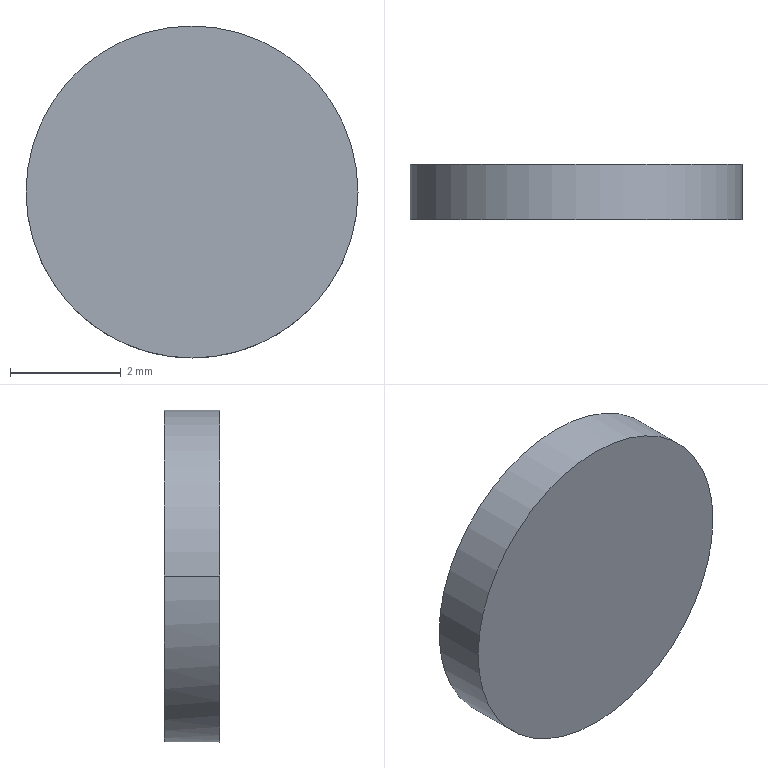Part | Creo | 1 solid | 17 faces | box 6 x 1 x 6 mm | volume 26.294 mm3 | plane 15 | cylinder 2 | commonest cylinder face diameters 6 x2
STEP:
#1=CARTESIAN_POINT('',(0.,0.,0.));
#2=DIRECTION('',(0.,0.,1.));
#3=DIRECTION('',(1.,0.,0.));
#4=AXIS2_PLACEMENT_3D('',#1,#2,#3);
#5=CARTESIAN_POINT('',(58.,52.,60.91));
#6=VERTEX_POINT('',#5);
#7=CARTESIAN_POINT('',(55.,52.,63.91));
#8=VERTEX_POINT('',#7);
#9=CARTESIAN_POINT('',(55.,52.,60.91));
#10=DIRECTION('',(0.,-1.,0.));
#11=DIRECTION('',(1.,0.,0.));
#12=AXIS2_PLACEMENT_3D('',#9,#10,#11);
#13=CIRCLE('',#12,3.);
#14=EDGE_CURVE('',#6,#8,#13,.T.);
#15=ORIENTED_EDGE('',*,*,#14,.T.);
#16=CARTESIAN_POINT('',(52.,52.,60.91));
#17=VERTEX_POINT('',#16);
#18=CARTESIAN_POINT('',(55.,52.,60.91));
#19=DIRECTION('',(0.,-1.,0.));
#20=DIRECTION('',(0.,0.,1.));
#21=AXIS2_PLACEMENT_3D('',#18,#19,#20);
#22=CIRCLE('',#21,3.);
#23=EDGE_CURVE('',#8,#17,#22,.T.);
#24=ORIENTED_EDGE('',*,*,#23,.T.);
#25=CARTESIAN_POINT('',(52.,53.,60.91));
#26=VERTEX_POINT('',#25);
#27=CARTESIAN_POINT('',(52.,52.,60.91));
#28=DIRECTION('',(0.,1.,0.));
#29=VECTOR('',#28,1.);
#30=LINE('',#27,#29);
#31=EDGE_CURVE('',#17,#26,#30,.T.);
#32=ORIENTED_EDGE('',*,*,#31,.T.);
#33=CARTESIAN_POINT('',(55.,53.,63.91));
#34=VERTEX_POINT('',#33);
#35=CARTESIAN_POINT('',(55.,53.,60.91));
#36=DIRECTION('',(0.,1.,0.));
#37=DIRECTION('',(-1.,0.,0.));
#38=AXIS2_PLACEMENT_3D('',#35,#36,#37);
#39=CIRCLE('',#38,3.);
#40=EDGE_CURVE('',#26,#34,#39,.T.);
#41=ORIENTED_EDGE('',*,*,#40,.T.);
#42=CARTESIAN_POINT('',(58.,53.,60.91));
#43=VERTEX_POINT('',#42);
#44=CARTESIAN_POINT('',(55.,53.,60.91));
#45=DIRECTION('',(0.,1.,0.));
#46=DIRECTION('',(0.,0.,1.));
#47=AXIS2_PLACEMENT_3D('',#44,#45,#46);
#48=CIRCLE('',#47,3.);
#49=EDGE_CURVE('',#34,#43,#48,.T.);
#50=ORIENTED_EDGE('',*,*,#49,.T.);
#51=CARTESIAN_POINT('',(58.,52.,60.91));
#52=DIRECTION('',(0.,1.,0.));
#53=VECTOR('',#52,1.);
#54=LINE('',#51,#53);
#55=EDGE_CURVE('',#6,#43,#54,.T.);
#56=ORIENTED_EDGE('',*,*,#55,.F.);
#57=EDGE_LOOP('',(#15,#24,#32,#41,#50,#56));
#58=FACE_OUTER_BOUND('',#57,.F.);
#59=CARTESIAN_POINT('',(55.,52.,60.91));
#60=DIRECTION('',(0.,1.,0.));
#61=DIRECTION('',(-1.,0.,0.));
#62=AXIS2_PLACEMENT_3D('',#59,#60,#61);
#63=CYLINDRICAL_SURFACE('',#62,3.);
#64=ADVANCED_FACE('',(#58),#63,.T.);
#65=ORIENTED_EDGE('',*,*,#23,.F.);
#66=ORIENTED_EDGE('',*,*,#14,.F.);
#67=CARTESIAN_POINT('',(55.,52.,57.91));
#68=VERTEX_POINT('',#67);
#69=CARTESIAN_POINT('',(55.,52.,60.91));
#70=DIRECTION('',(0.,-1.,0.));
#71=DIRECTION('',(0.,0.,-1.));
#72=AXIS2_PLACEMENT_3D('',#69,#70,#71);
#73=CIRCLE('',#72,3.);
#74=EDGE_CURVE('',#68,#6,#73,.T.);
#75=ORIENTED_EDGE('',*,*,#74,.F.);
#76=CARTESIAN_POINT('',(55.,52.,60.91));
#77=DIRECTION('',(0.,-1.,0.));
#78=DIRECTION('',(-1.,0.,0.));
#79=AXIS2_PLACEMENT_3D('',#76,#77,#78);
#80=CIRCLE('',#79,3.);
#81=EDGE_CURVE('',#17,#68,#80,.T.);
#82=ORIENTED_EDGE('',*,*,#81,.F.);
#83=EDGE_LOOP('',(#65,#66,#75,#82));
#84=FACE_OUTER_BOUND('',#83,.F.);
#85=CARTESIAN_POINT('',(55.,52.,60.91));
#86=DIRECTION('',(0.,-1.,0.));
#87=DIRECTION('',(1.,0.,0.));
#88=AXIS2_PLACEMENT_3D('',#85,#86,#87);
#89=PLANE('',#88);
#90=ADVANCED_FACE('',(#84),#89,.T.);
#91=ORIENTED_EDGE('',*,*,#74,.T.);
#92=ORIENTED_EDGE('',*,*,#55,.T.);
#93=CARTESIAN_POINT('',(55.,53.,60.91));
#94=DIRECTION('',(0.,1.,0.));
#95=DIRECTION('',(1.,0.,0.));
#96=AXIS2_PLACEMENT_3D('',#93,#94,#95);
#97=CIRCLE('',#96,3.);
#98=EDGE_CURVE('',#43,#26,#97,.T.);
#99=ORIENTED_EDGE('',*,*,#98,.T.);
#100=ORIENTED_EDGE('',*,*,#31,.F.);
#101=ORIENTED_EDGE('',*,*,#81,.T.);
#102=EDGE_LOOP('',(#91,#92,#99,#100,#101));
#103=FACE_OUTER_BOUND('',#102,.F.);
#104=CARTESIAN_POINT('',(55.,52.,60.91));
#105=DIRECTION('',(0.,1.,0.));
#106=DIRECTION('',(-1.,0.,0.));
#107=AXIS2_PLACEMENT_3D('',#104,#105,#106);
#108=CYLINDRICAL_SURFACE('',#107,3.);
#109=ADVANCED_FACE('',(#103),#108,.T.);
#110=ORIENTED_EDGE('',*,*,#49,.F.);
#111=ORIENTED_EDGE('',*,*,#40,.F.);
#112=ORIENTED_EDGE('',*,*,#98,.F.);
#113=EDGE_LOOP('',(#110,#111,#112));
#114=FACE_OUTER_BOUND('',#113,.F.);
#115=CARTESIAN_POINT('',(53.2,53.,61.21));
#116=VERTEX_POINT('',#115);
#117=CARTESIAN_POINT('',(54.7,53.,61.21));
#118=VERTEX_POINT('',#117);
#119=CARTESIAN_POINT('',(53.2,53.,61.21));
#120=DIRECTION('',(1.,0.,0.));
#121=VECTOR('',#120,1.5);
#122=LINE('',#119,#121);
#123=EDGE_CURVE('',#116,#118,#122,.T.);
#124=ORIENTED_EDGE('',*,*,#123,.T.);
#125=CARTESIAN_POINT('',(54.7,53.,62.71));
#126=VERTEX_POINT('',#125);
#127=CARTESIAN_POINT('',(54.7,53.,61.21));
#128=DIRECTION('',(0.,0.,1.));
#129=VECTOR('',#128,1.5);
#130=LINE('',#127,#129);
#131=EDGE_CURVE('',#118,#126,#130,.T.);
#132=ORIENTED_EDGE('',*,*,#131,.T.);
#133=CARTESIAN_POINT('',(55.3,53.,62.71));
#134=VERTEX_POINT('',#133);
#135=CARTESIAN_POINT('',(54.7,53.,62.71));
#136=DIRECTION('',(1.,0.,0.));
#137=VECTOR('',#136,0.6);
#138=LINE('',#135,#137);
#139=EDGE_CURVE('',#126,#134,#138,.T.);
#140=ORIENTED_EDGE('',*,*,#139,.T.);
#141=CARTESIAN_POINT('',(55.3,53.,61.21));
#142=VERTEX_POINT('',#141);
#143=CARTESIAN_POINT('',(55.3,53.,62.71));
#144=DIRECTION('',(0.,0.,-1.));
#145=VECTOR('',#144,1.5);
#146=LINE('',#143,#145);
#147=EDGE_CURVE('',#134,#142,#146,.T.);
#148=ORIENTED_EDGE('',*,*,#147,.T.);
#149=CARTESIAN_POINT('',(56.8,53.,61.21));
#150=VERTEX_POINT('',#149);
#151=CARTESIAN_POINT('',(55.3,53.,61.21));
#152=DIRECTION('',(1.,0.,0.));
#153=VECTOR('',#152,1.5);
#154=LINE('',#151,#153);
#155=EDGE_CURVE('',#142,#150,#154,.T.);
#156=ORIENTED_EDGE('',*,*,#155,.T.);
#157=CARTESIAN_POINT('',(56.8,53.,60.61));
#158=VERTEX_POINT('',#157);
#159=CARTESIAN_POINT('',(56.8,53.,61.21));
#160=DIRECTION('',(0.,0.,-1.));
#161=VECTOR('',#160,0.6);
#162=LINE('',#159,#161);
#163=EDGE_CURVE('',#150,#158,#162,.T.);
#164=ORIENTED_EDGE('',*,*,#163,.T.);
#165=CARTESIAN_POINT('',(55.3,53.,60.61));
#166=VERTEX_POINT('',#165);
#167=CARTESIAN_POINT('',(56.8,53.,60.61));
#168=DIRECTION('',(-1.,0.,0.));
#169=VECTOR('',#168,1.5);
#170=LINE('',#167,#169);
#171=EDGE_CURVE('',#158,#166,#170,.T.);
#172=ORIENTED_EDGE('',*,*,#171,.T.);
#173=CARTESIAN_POINT('',(55.3,53.,59.11));
#174=VERTEX_POINT('',#173);
#175=CARTESIAN_POINT('',(55.3,53.,60.61));
#176=DIRECTION('',(0.,0.,-1.));
#177=VECTOR('',#176,1.5);
#178=LINE('',#175,#177);
#179=EDGE_CURVE('',#166,#174,#178,.T.);
#180=ORIENTED_EDGE('',*,*,#179,.T.);
#181=CARTESIAN_POINT('',(54.7,53.,59.11));
#182=VERTEX_POINT('',#181);
#183=CARTESIAN_POINT('',(55.3,53.,59.11));
#184=DIRECTION('',(-1.,0.,0.));
#185=VECTOR('',#184,0.6);
#186=LINE('',#183,#185);
#187=EDGE_CURVE('',#174,#182,#186,.T.);
#188=ORIENTED_EDGE('',*,*,#187,.T.);
#189=CARTESIAN_POINT('',(54.7,53.,60.61));
#190=VERTEX_POINT('',#189);
#191=CARTESIAN_POINT('',(54.7,53.,59.11));
#192=DIRECTION('',(0.,0.,1.));
#193=VECTOR('',#192,1.5);
#194=LINE('',#191,#193);
#195=EDGE_CURVE('',#182,#190,#194,.T.);
#196=ORIENTED_EDGE('',*,*,#195,.T.);
#197=CARTESIAN_POINT('',(53.2,53.,60.61));
#198=VERTEX_POINT('',#197);
#199=CARTESIAN_POINT('',(54.7,53.,60.61));
#200=DIRECTION('',(-1.,0.,0.));
#201=VECTOR('',#200,1.5);
#202=LINE('',#199,#201);
#203=EDGE_CURVE('',#190,#198,#202,.T.);
#204=ORIENTED_EDGE('',*,*,#203,.T.);
#205=CARTESIAN_POINT('',(53.2,53.,60.61));
#206=DIRECTION('',(0.,0.,1.));
#207=VECTOR('',#206,0.6);
#208=LINE('',#205,#207);
#209=EDGE_CURVE('',#198,#116,#208,.T.);
#210=ORIENTED_EDGE('',*,*,#209,.T.);
#211=EDGE_LOOP('',(#124,#132,#140,#148,#156,#164,#172,#180,#188,#196,#204,#210));
#212=FACE_BOUND('',#211,.F.);
#213=CARTESIAN_POINT('',(55.,53.,60.91));
#214=DIRECTION('',(0.,-1.,0.));
#215=DIRECTION('',(1.,0.,0.));
#216=AXIS2_PLACEMENT_3D('',#213,#214,#215);
#217=PLANE('',#216);
#218=ADVANCED_FACE('',(#114,#212),#217,.F.);
#219=ORIENTED_EDGE('',*,*,#123,.F.);
#220=CARTESIAN_POINT('',(53.2,52.5,61.21));
#221=VERTEX_POINT('',#220);
#222=CARTESIAN_POINT('',(53.2,52.5,61.21));
#223=DIRECTION('',(0.,1.,0.));
#224=VECTOR('',#223,0.5);
#225=LINE('',#222,#224);
#226=EDGE_CURVE('',#221,#116,#225,.T.);
#227=ORIENTED_EDGE('',*,*,#226,.F.);
#228=CARTESIAN_POINT('',(54.7,52.5,61.21));
#229=VERTEX_POINT('',#228);
#230=CARTESIAN_POINT('',(54.7,52.5,61.21));
#231=DIRECTION('',(-1.,0.,0.));
#232=VECTOR('',#231,1.5);
#233=LINE('',#230,#232);
#234=EDGE_CURVE('',#229,#221,#233,.T.);
#235=ORIENTED_EDGE('',*,*,#234,.F.);
#236=CARTESIAN_POINT('',(54.7,52.5,61.21));
#237=DIRECTION('',(0.,1.,0.));
#238=VECTOR('',#237,0.5);
#239=LINE('',#236,#238);
#240=EDGE_CURVE('',#229,#118,#239,.T.);
#241=ORIENTED_EDGE('',*,*,#240,.T.);
#242=EDGE_LOOP('',(#219,#227,#235,#241));
#243=FACE_OUTER_BOUND('',#242,.F.);
#244=CARTESIAN_POINT('',(54.7,52.5,61.21));
#245=DIRECTION('',(0.,0.,-1.));
#246=DIRECTION('',(-1.,0.,0.));
#247=AXIS2_PLACEMENT_3D('',#244,#245,#246);
#248=PLANE('',#247);
#249=ADVANCED_FACE('',(#243),#248,.T.);
#250=ORIENTED_EDGE('',*,*,#209,.F.);
#251=CARTESIAN_POINT('',(53.2,52.5,60.61));
#252=VERTEX_POINT('',#251);
#253=CARTESIAN_POINT('',(53.2,52.5,60.61));
#254=DIRECTION('',(0.,1.,0.));
#255=VECTOR('',#254,0.5);
#256=LINE('',#253,#255);
#257=EDGE_CURVE('',#252,#198,#256,.T.);
#258=ORIENTED_EDGE('',*,*,#257,.F.);
#259=CARTESIAN_POINT('',(53.2,52.5,61.21));
#260=DIRECTION('',(0.,0.,-1.));
#261=VECTOR('',#260,0.6);
#262=LINE('',#259,#261);
#263=EDGE_CURVE('',#221,#252,#262,.T.);
#264=ORIENTED_EDGE('',*,*,#263,.F.);
#265=ORIENTED_EDGE('',*,*,#226,.T.);
#266=EDGE_LOOP('',(#250,#258,#264,#265));
#267=FACE_OUTER_BOUND('',#266,.F.);
#268=CARTESIAN_POINT('',(53.2,52.5,61.21));
#269=DIRECTION('',(1.,0.,0.));
#270=DIRECTION('',(0.,1.,0.));
#271=AXIS2_PLACEMENT_3D('',#268,#269,#270);
#272=PLANE('',#271);
#273=ADVANCED_FACE('',(#267),#272,.T.);
#274=ORIENTED_EDGE('',*,*,#203,.F.);
#275=CARTESIAN_POINT('',(54.7,52.5,60.61));
#276=VERTEX_POINT('',#275);
#277=CARTESIAN_POINT('',(54.7,52.5,60.61));
#278=DIRECTION('',(0.,1.,0.));
#279=VECTOR('',#278,0.5);
#280=LINE('',#277,#279);
#281=EDGE_CURVE('',#276,#190,#280,.T.);
#282=ORIENTED_EDGE('',*,*,#281,.F.);
#283=CARTESIAN_POINT('',(53.2,52.5,60.61));
#284=DIRECTION('',(1.,0.,0.));
#285=VECTOR('',#284,1.5);
#286=LINE('',#283,#285);
#287=EDGE_CURVE('',#252,#276,#286,.T.);
#288=ORIENTED_EDGE('',*,*,#287,.F.);
#289=ORIENTED_EDGE('',*,*,#257,.T.);
#290=EDGE_LOOP('',(#274,#282,#288,#289));
#291=FACE_OUTER_BOUND('',#290,.F.);
#292=CARTESIAN_POINT('',(53.2,52.5,60.61));
#293=DIRECTION('',(0.,0.,1.));
#294=DIRECTION('',(1.,0.,0.));
#295=AXIS2_PLACEMENT_3D('',#292,#293,#294);
#296=PLANE('',#295);
#297=ADVANCED_FACE('',(#291),#296,.T.);
#298=ORIENTED_EDGE('',*,*,#195,.F.);
#299=CARTESIAN_POINT('',(54.7,52.5,59.11));
#300=VERTEX_POINT('',#299);
#301=CARTESIAN_POINT('',(54.7,52.5,59.11));
#302=DIRECTION('',(0.,1.,0.));
#303=VECTOR('',#302,0.5);
#304=LINE('',#301,#303);
#305=EDGE_CURVE('',#300,#182,#304,.T.);
#306=ORIENTED_EDGE('',*,*,#305,.F.);
#307=CARTESIAN_POINT('',(54.7,52.5,60.61));
#308=DIRECTION('',(0.,0.,-1.));
#309=VECTOR('',#308,1.5);
#310=LINE('',#307,#309);
#311=EDGE_CURVE('',#276,#300,#310,.T.);
#312=ORIENTED_EDGE('',*,*,#311,.F.);
#313=ORIENTED_EDGE('',*,*,#281,.T.);
#314=EDGE_LOOP('',(#298,#306,#312,#313));
#315=FACE_OUTER_BOUND('',#314,.F.);
#316=CARTESIAN_POINT('',(54.7,52.5,60.61));
#317=DIRECTION('',(1.,0.,0.));
#318=DIRECTION('',(0.,0.,-1.));
#319=AXIS2_PLACEMENT_3D('',#316,#317,#318);
#320=PLANE('',#319);
#321=ADVANCED_FACE('',(#315),#320,.T.);
#322=ORIENTED_EDGE('',*,*,#187,.F.);
#323=CARTESIAN_POINT('',(55.3,52.5,59.11));
#324=VERTEX_POINT('',#323);
#325=CARTESIAN_POINT('',(55.3,52.5,59.11));
#326=DIRECTION('',(0.,1.,0.));
#327=VECTOR('',#326,0.5);
#328=LINE('',#325,#327);
#329=EDGE_CURVE('',#324,#174,#328,.T.);
#330=ORIENTED_EDGE('',*,*,#329,.F.);
#331=CARTESIAN_POINT('',(54.7,52.5,59.11));
#332=DIRECTION('',(1.,0.,0.));
#333=VECTOR('',#332,0.6);
#334=LINE('',#331,#333);
#335=EDGE_CURVE('',#300,#324,#334,.T.);
#336=ORIENTED_EDGE('',*,*,#335,.F.);
#337=ORIENTED_EDGE('',*,*,#305,.T.);
#338=EDGE_LOOP('',(#322,#330,#336,#337));
#339=FACE_OUTER_BOUND('',#338,.F.);
#340=CARTESIAN_POINT('',(54.7,52.5,59.11));
#341=DIRECTION('',(0.,0.,1.));
#342=DIRECTION('',(0.,1.,0.));
#343=AXIS2_PLACEMENT_3D('',#340,#341,#342);
#344=PLANE('',#343);
#345=ADVANCED_FACE('',(#339),#344,.T.);
#346=ORIENTED_EDGE('',*,*,#179,.F.);
#347=CARTESIAN_POINT('',(55.3,52.5,60.61));
#348=VERTEX_POINT('',#347);
#349=CARTESIAN_POINT('',(55.3,52.5,60.61));
#350=DIRECTION('',(0.,1.,0.));
#351=VECTOR('',#350,0.5);
#352=LINE('',#349,#351);
#353=EDGE_CURVE('',#348,#166,#352,.T.);
#354=ORIENTED_EDGE('',*,*,#353,.F.);
#355=CARTESIAN_POINT('',(55.3,52.5,59.11));
#356=DIRECTION('',(0.,0.,1.));
#357=VECTOR('',#356,1.5);
#358=LINE('',#355,#357);
#359=EDGE_CURVE('',#324,#348,#358,.T.);
#360=ORIENTED_EDGE('',*,*,#359,.F.);
#361=ORIENTED_EDGE('',*,*,#329,.T.);
#362=EDGE_LOOP('',(#346,#354,#360,#361));
#363=FACE_OUTER_BOUND('',#362,.F.);
#364=CARTESIAN_POINT('',(55.3,52.5,59.11));
#365=DIRECTION('',(-1.,0.,0.));
#366=DIRECTION('',(0.,0.,1.));
#367=AXIS2_PLACEMENT_3D('',#364,#365,#366);
#368=PLANE('',#367);
#369=ADVANCED_FACE('',(#363),#368,.T.);
#370=ORIENTED_EDGE('',*,*,#171,.F.);
#371=CARTESIAN_POINT('',(56.8,52.5,60.61));
#372=VERTEX_POINT('',#371);
#373=CARTESIAN_POINT('',(56.8,52.5,60.61));
#374=DIRECTION('',(0.,1.,0.));
#375=VECTOR('',#374,0.5);
#376=LINE('',#373,#375);
#377=EDGE_CURVE('',#372,#158,#376,.T.);
#378=ORIENTED_EDGE('',*,*,#377,.F.);
#379=CARTESIAN_POINT('',(55.3,52.5,60.61));
#380=DIRECTION('',(1.,0.,0.));
#381=VECTOR('',#380,1.5);
#382=LINE('',#379,#381);
#383=EDGE_CURVE('',#348,#372,#382,.T.);
#384=ORIENTED_EDGE('',*,*,#383,.F.);
#385=ORIENTED_EDGE('',*,*,#353,.T.);
#386=EDGE_LOOP('',(#370,#378,#384,#385));
#387=FACE_OUTER_BOUND('',#386,.F.);
#388=CARTESIAN_POINT('',(55.3,52.5,60.61));
#389=DIRECTION('',(0.,0.,1.));
#390=DIRECTION('',(1.,0.,0.));
#391=AXIS2_PLACEMENT_3D('',#388,#389,#390);
#392=PLANE('',#391);
#393=ADVANCED_FACE('',(#387),#392,.T.);
#394=ORIENTED_EDGE('',*,*,#163,.F.);
#395=CARTESIAN_POINT('',(56.8,52.5,61.21));
#396=VERTEX_POINT('',#395);
#397=CARTESIAN_POINT('',(56.8,52.5,61.21));
#398=DIRECTION('',(0.,1.,0.));
#399=VECTOR('',#398,0.5);
#400=LINE('',#397,#399);
#401=EDGE_CURVE('',#396,#150,#400,.T.);
#402=ORIENTED_EDGE('',*,*,#401,.F.);
#403=CARTESIAN_POINT('',(56.8,52.5,60.61));
#404=DIRECTION('',(0.,0.,1.));
#405=VECTOR('',#404,0.6);
#406=LINE('',#403,#405);
#407=EDGE_CURVE('',#372,#396,#406,.T.);
#408=ORIENTED_EDGE('',*,*,#407,.F.);
#409=ORIENTED_EDGE('',*,*,#377,.T.);
#410=EDGE_LOOP('',(#394,#402,#408,#409));
#411=FACE_OUTER_BOUND('',#410,.F.);
#412=CARTESIAN_POINT('',(56.8,52.5,60.61));
#413=DIRECTION('',(-1.,0.,0.));
#414=DIRECTION('',(0.,-1.,0.));
#415=AXIS2_PLACEMENT_3D('',#412,#413,#414);
#416=PLANE('',#415);
#417=ADVANCED_FACE('',(#411),#416,.T.);
#418=ORIENTED_EDGE('',*,*,#155,.F.);
#419=CARTESIAN_POINT('',(55.3,52.5,61.21));
#420=VERTEX_POINT('',#419);
#421=CARTESIAN_POINT('',(55.3,52.5,61.21));
#422=DIRECTION('',(0.,1.,0.));
#423=VECTOR('',#422,0.5);
#424=LINE('',#421,#423);
#425=EDGE_CURVE('',#420,#142,#424,.T.);
#426=ORIENTED_EDGE('',*,*,#425,.F.);
#427=CARTESIAN_POINT('',(56.8,52.5,61.21));
#428=DIRECTION('',(-1.,0.,0.));
#429=VECTOR('',#428,1.5);
#430=LINE('',#427,#429);
#431=EDGE_CURVE('',#396,#420,#430,.T.);
#432=ORIENTED_EDGE('',*,*,#431,.F.);
#433=ORIENTED_EDGE('',*,*,#401,.T.);
#434=EDGE_LOOP('',(#418,#426,#432,#433));
#435=FACE_OUTER_BOUND('',#434,.F.);
#436=CARTESIAN_POINT('',(56.8,52.5,61.21));
#437=DIRECTION('',(0.,0.,-1.));
#438=DIRECTION('',(-1.,0.,0.));
#439=AXIS2_PLACEMENT_3D('',#436,#437,#438);
#440=PLANE('',#439);
#441=ADVANCED_FACE('',(#435),#440,.T.);
#442=ORIENTED_EDGE('',*,*,#147,.F.);
#443=CARTESIAN_POINT('',(55.3,52.5,62.71));
#444=VERTEX_POINT('',#443);
#445=CARTESIAN_POINT('',(55.3,52.5,62.71));
#446=DIRECTION('',(0.,1.,0.));
#447=VECTOR('',#446,0.5);
#448=LINE('',#445,#447);
#449=EDGE_CURVE('',#444,#134,#448,.T.);
#450=ORIENTED_EDGE('',*,*,#449,.F.);
#451=CARTESIAN_POINT('',(55.3,52.5,61.21));
#452=DIRECTION('',(0.,0.,1.));
#453=VECTOR('',#452,1.5);
#454=LINE('',#451,#453);
#455=EDGE_CURVE('',#420,#444,#454,.T.);
#456=ORIENTED_EDGE('',*,*,#455,.F.);
#457=ORIENTED_EDGE('',*,*,#425,.T.);
#458=EDGE_LOOP('',(#442,#450,#456,#457));
#459=FACE_OUTER_BOUND('',#458,.F.);
#460=CARTESIAN_POINT('',(55.3,52.5,61.21));
#461=DIRECTION('',(-1.,0.,0.));
#462=DIRECTION('',(0.,0.,1.));
#463=AXIS2_PLACEMENT_3D('',#460,#461,#462);
#464=PLANE('',#463);
#465=ADVANCED_FACE('',(#459),#464,.T.);
#466=ORIENTED_EDGE('',*,*,#139,.F.);
#467=CARTESIAN_POINT('',(54.7,52.5,62.71));
#468=VERTEX_POINT('',#467);
#469=CARTESIAN_POINT('',(54.7,52.5,62.71));
#470=DIRECTION('',(0.,1.,0.));
#471=VECTOR('',#470,0.5);
#472=LINE('',#469,#471);
#473=EDGE_CURVE('',#468,#126,#472,.T.);
#474=ORIENTED_EDGE('',*,*,#473,.F.);
#475=CARTESIAN_POINT('',(55.3,52.5,62.71));
#476=DIRECTION('',(-1.,0.,0.));
#477=VECTOR('',#476,0.6);
#478=LINE('',#475,#477);
#479=EDGE_CURVE('',#444,#468,#478,.T.);
#480=ORIENTED_EDGE('',*,*,#479,.F.);
#481=ORIENTED_EDGE('',*,*,#449,.T.);
#482=EDGE_LOOP('',(#466,#474,#480,#481));
#483=FACE_OUTER_BOUND('',#482,.F.);
#484=CARTESIAN_POINT('',(55.3,52.5,62.71));
#485=DIRECTION('',(0.,0.,-1.));
#486=DIRECTION('',(0.,-1.,0.));
#487=AXIS2_PLACEMENT_3D('',#484,#485,#486);
#488=PLANE('',#487);
#489=ADVANCED_FACE('',(#483),#488,.T.);
#490=ORIENTED_EDGE('',*,*,#131,.F.);
#491=ORIENTED_EDGE('',*,*,#240,.F.);
#492=CARTESIAN_POINT('',(54.7,52.5,62.71));
#493=DIRECTION('',(0.,0.,-1.));
#494=VECTOR('',#493,1.5);
#495=LINE('',#492,#494);
#496=EDGE_CURVE('',#468,#229,#495,.T.);
#497=ORIENTED_EDGE('',*,*,#496,.F.);
#498=ORIENTED_EDGE('',*,*,#473,.T.);
#499=EDGE_LOOP('',(#490,#491,#497,#498));
#500=FACE_OUTER_BOUND('',#499,.F.);
#501=CARTESIAN_POINT('',(54.7,52.5,62.71));
#502=DIRECTION('',(1.,0.,0.));
#503=DIRECTION('',(0.,0.,-1.));
#504=AXIS2_PLACEMENT_3D('',#501,#502,#503);
#505=PLANE('',#504);
#506=ADVANCED_FACE('',(#500),#505,.T.);
#507=ORIENTED_EDGE('',*,*,#263,.T.);
#508=ORIENTED_EDGE('',*,*,#287,.T.);
#509=ORIENTED_EDGE('',*,*,#311,.T.);
#510=ORIENTED_EDGE('',*,*,#335,.T.);
#511=ORIENTED_EDGE('',*,*,#359,.T.);
#512=ORIENTED_EDGE('',*,*,#383,.T.);
#513=ORIENTED_EDGE('',*,*,#407,.T.);
#514=ORIENTED_EDGE('',*,*,#431,.T.);
#515=ORIENTED_EDGE('',*,*,#455,.T.);
#516=ORIENTED_EDGE('',*,*,#479,.T.);
#517=ORIENTED_EDGE('',*,*,#496,.T.);
#518=ORIENTED_EDGE('',*,*,#234,.T.);
#519=EDGE_LOOP('',(#507,#508,#509,#510,#511,#512,#513,#514,#515,#516,#517,#518));
#520=FACE_OUTER_BOUND('',#519,.F.);
#521=CARTESIAN_POINT('',(55.,52.5,60.91));
#522=DIRECTION('',(0.,-1.,0.));
#523=DIRECTION('',(1.,0.,0.));
#524=AXIS2_PLACEMENT_3D('',#521,#522,#523);
#525=PLANE('',#524);
#526=ADVANCED_FACE('',(#520),#525,.F.);
#527=CLOSED_SHELL('',(#64,#90,#109,#218,#249,#273,#297,#321,#345,#369,#393,#417,#441,#465,#489,#506,#526));
#528=MANIFOLD_SOLID_BREP('',#527);
#529=(LENGTH_UNIT()NAMED_UNIT(*)SI_UNIT(.MILLI.,.METRE.));
#530=UNCERTAINTY_MEASURE_WITH_UNIT(LENGTH_MEASURE(0.0008545),#529,'','');
#531=(NAMED_UNIT(*)PLANE_ANGLE_UNIT()SI_UNIT($,.RADIAN.));
#532=PLANE_ANGLE_MEASURE_WITH_UNIT(PLANE_ANGLE_MEASURE(0.01745),#531);
#533=(CONVERSION_BASED_UNIT('DEGREE',#532)NAMED_UNIT(*)PLANE_ANGLE_UNIT());
#534=(NAMED_UNIT(*)SI_UNIT($,.STERADIAN.)SOLID_ANGLE_UNIT());
#535=(GEOMETRIC_REPRESENTATION_CONTEXT(3)GLOBAL_UNCERTAINTY_ASSIGNED_CONTEXT((#530))GLOBAL_UNIT_ASSIGNED_CONTEXT((#529,#533,#534))REPRESENTATION_CONTEXT('',''));
#536=ADVANCED_BREP_SHAPE_REPRESENTATION('',(#4,#528),#535);